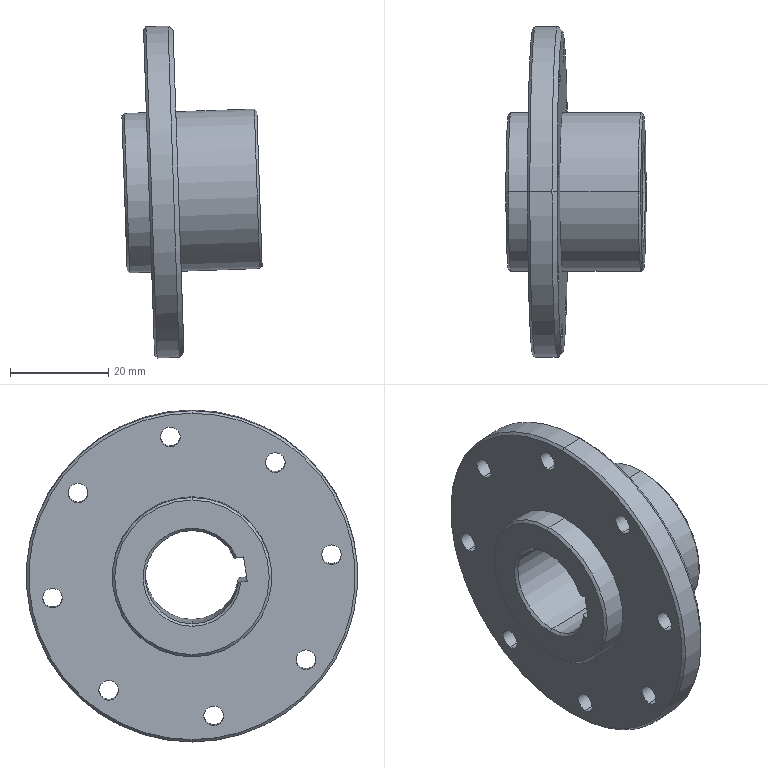Part | STEP file | 2026.6.15-Main Assembly图.sldasm-Part-101 | 1 solid | 46 faces | box 28.549 x 67.5 x 67.614 mm | volume 30514 mm3 | cylinder 25 | cone 14 | plane 7 | commonest cylinder face diameters 4 x16 32.5 x4 19 x3 67.5 x2
STEP:
#1=CARTESIAN_POINT('',(-1623.534,735.086,4084.159));
#2=VERTEX_POINT('',#1);
#3=CARTESIAN_POINT('',(-1625.749,735.086,4149.621));
#4=VERTEX_POINT('',#3);
#5=CARTESIAN_POINT('',(-1624.641,735.086,4116.89));
#6=DIRECTION('',(0.9994,0.,0.03381));
#7=DIRECTION('',(0.03381,0.,-0.9994));
#8=AXIS2_PLACEMENT_3D('',#5,#6,#7);
#9=CIRCLE('',#8,32.75);
#10=EDGE_CURVE('',#2,#4,#9,.T.);
#11=ORIENTED_EDGE('',*,*,#10,.F.);
#12=CARTESIAN_POINT('',(-1624.499,735.086,4083.125));
#13=VERTEX_POINT('',#12);
#14=CARTESIAN_POINT('',(-1623.534,735.086,4084.159));
#15=DIRECTION('',(-0.6828,0.,-0.7306));
#16=VECTOR('',#15,1000.);
#17=LINE('',#14,#16);
#18=EDGE_CURVE('',#2,#13,#17,.T.);
#19=ORIENTED_EDGE('',*,*,#18,.T.);
#20=CARTESIAN_POINT('',(-1626.782,735.086,4150.587));
#21=VERTEX_POINT('',#20);
#22=CARTESIAN_POINT('',(-1625.641,735.086,4116.856));
#23=DIRECTION('',(-0.9994,0.,-0.03381));
#24=DIRECTION('',(0.03381,0.,-0.9994));
#25=AXIS2_PLACEMENT_3D('',#22,#23,#24);
#26=CIRCLE('',#25,33.75);
#27=EDGE_CURVE('',#21,#13,#26,.T.);
#28=ORIENTED_EDGE('',*,*,#27,.F.);
#29=CARTESIAN_POINT('',(-1625.749,735.086,4149.621));
#30=DIRECTION('',(-0.7306,0.,0.6828));
#31=VECTOR('',#30,1000.);
#32=LINE('',#29,#31);
#33=EDGE_CURVE('',#4,#21,#32,.T.);
#34=ORIENTED_EDGE('',*,*,#33,.F.);
#35=EDGE_LOOP('',(#11,#19,#28,#34));
#36=FACE_OUTER_BOUND('',#35,.T.);
#37=CARTESIAN_POINT('',(-1624.641,735.086,4116.89));
#38=DIRECTION('',(-0.9994,0.,-0.03381));
#39=DIRECTION('',(-0.03381,0.,0.9994));
#40=AXIS2_PLACEMENT_3D('',#37,#38,#39);
#41=CONICAL_SURFACE('',#40,32.75,0.7854);
#42=ADVANCED_FACE('',(#36),#41,.T.);
#43=CARTESIAN_POINT('',(-1634.814,735.086,4107.04));
#44=VERTEX_POINT('',#43);
#45=CARTESIAN_POINT('',(-1635.099,725.645,4115.472));
#46=VERTEX_POINT('',#45);
#47=CARTESIAN_POINT('',(-1635.135,735.086,4116.535));
#48=DIRECTION('',(-0.9994,0.,-0.03381));
#49=DIRECTION('',(0.03381,0.,-0.9994));
#50=AXIS2_PLACEMENT_3D('',#47,#48,#49);
#51=CIRCLE('',#50,9.5);
#52=EDGE_CURVE('',#44,#46,#51,.T.);
#53=ORIENTED_EDGE('',*,*,#52,.F.);
#54=CARTESIAN_POINT('',(-1635.297,735.086,4106.524));
#55=VERTEX_POINT('',#54);
#56=CARTESIAN_POINT('',(-1634.814,735.086,4107.04));
#57=DIRECTION('',(-0.6828,0.,-0.7306));
#58=VECTOR('',#57,1000.);
#59=LINE('',#56,#58);
#60=EDGE_CURVE('',#44,#55,#59,.T.);
#61=ORIENTED_EDGE('',*,*,#60,.T.);
#62=CARTESIAN_POINT('',(-1635.602,725.134,4115.534));
#63=VERTEX_POINT('',#62);
#64=CARTESIAN_POINT('',(-1635.635,735.086,4116.518));
#65=DIRECTION('',(0.9994,0.,0.03381));
#66=DIRECTION('',(0.03381,0.,-0.9994));
#67=AXIS2_PLACEMENT_3D('',#64,#65,#66);
#68=CIRCLE('',#67,10.);
#69=EDGE_CURVE('',#63,#55,#68,.T.);
#70=ORIENTED_EDGE('',*,*,#69,.F.);
#71=CARTESIAN_POINT('',(-1635.099,725.645,4115.472));
#72=CARTESIAN_POINT('',(-1635.267,725.475,4115.493));
#73=CARTESIAN_POINT('',(-1635.434,725.305,4115.513));
#74=CARTESIAN_POINT('',(-1635.602,725.134,4115.534));
#75=B_SPLINE_CURVE_WITH_KNOTS('',3,(#71,#72,#73,#74),.UNSPECIFIED.,.F.,.F.,(4,4),(0.,0.0007194),.UNSPECIFIED.);
#76=EDGE_CURVE('',#46,#63,#75,.T.);
#77=ORIENTED_EDGE('',*,*,#76,.F.);
#78=EDGE_LOOP('',(#53,#61,#70,#77));
#79=FACE_OUTER_BOUND('',#78,.T.);
#80=CARTESIAN_POINT('',(-1635.135,735.086,4116.535));
#81=DIRECTION('',(-0.9994,0.,-0.03381));
#82=DIRECTION('',(-0.03381,0.,0.9994));
#83=AXIS2_PLACEMENT_3D('',#80,#81,#82);
#84=CONICAL_SURFACE('',#83,9.5,0.7854);
#85=ADVANCED_FACE('',(#79),#84,.F.);
#86=ORIENTED_EDGE('',*,*,#60,.F.);
#87=CARTESIAN_POINT('',(-1635.457,735.086,4126.03));
#88=VERTEX_POINT('',#87);
#89=CARTESIAN_POINT('',(-1635.135,735.086,4116.535));
#90=DIRECTION('',(-0.9994,0.,-0.03381));
#91=DIRECTION('',(0.03381,0.,-0.9994));
#92=AXIS2_PLACEMENT_3D('',#89,#90,#91);
#93=CIRCLE('',#92,9.5);
#94=EDGE_CURVE('',#88,#44,#93,.T.);
#95=ORIENTED_EDGE('',*,*,#94,.F.);
#96=CARTESIAN_POINT('',(-1635.973,735.086,4126.512));
#97=VERTEX_POINT('',#96);
#98=CARTESIAN_POINT('',(-1635.457,735.086,4126.03));
#99=DIRECTION('',(-0.7306,0.,0.6828));
#100=VECTOR('',#99,1000.);
#101=LINE('',#98,#100);
#102=EDGE_CURVE('',#88,#97,#101,.T.);
#103=ORIENTED_EDGE('',*,*,#102,.T.);
#104=CARTESIAN_POINT('',(-1635.635,735.086,4116.518));
#105=DIRECTION('',(0.9994,0.,0.03381));
#106=DIRECTION('',(0.03381,0.,-0.9994));
#107=AXIS2_PLACEMENT_3D('',#104,#105,#106);
#108=CIRCLE('',#107,10.);
#109=EDGE_CURVE('',#55,#97,#108,.T.);
#110=ORIENTED_EDGE('',*,*,#109,.F.);
#111=EDGE_LOOP('',(#86,#95,#103,#110));
#112=FACE_OUTER_BOUND('',#111,.T.);
#113=CARTESIAN_POINT('',(-1635.135,735.086,4116.535));
#114=DIRECTION('',(-0.9994,0.,-0.03381));
#115=DIRECTION('',(-0.03381,0.,0.9994));
#116=AXIS2_PLACEMENT_3D('',#113,#114,#115);
#117=CONICAL_SURFACE('',#116,9.5,0.7854);
#118=ADVANCED_FACE('',(#112),#117,.F.);
#119=CARTESIAN_POINT('',(-1636.168,735.086,4132.259));
#120=VERTEX_POINT('',#119);
#121=CARTESIAN_POINT('',(-1635.102,735.086,4100.777));
#122=VERTEX_POINT('',#121);
#123=CARTESIAN_POINT('',(-1635.635,735.086,4116.518));
#124=DIRECTION('',(-0.9994,0.,-0.03381));
#125=DIRECTION('',(0.03381,0.,-0.9994));
#126=AXIS2_PLACEMENT_3D('',#123,#124,#125);
#127=CIRCLE('',#126,15.75);
#128=EDGE_CURVE('',#120,#122,#127,.T.);
#129=ORIENTED_EDGE('',*,*,#128,.F.);
#130=CARTESIAN_POINT('',(-1635.685,735.086,4132.776));
#131=VERTEX_POINT('',#130);
#132=CARTESIAN_POINT('',(-1635.685,735.086,4132.776));
#133=DIRECTION('',(0.6828,0.,0.7306));
#134=VECTOR('',#133,1000.);
#135=LINE('',#132,#134);
#136=EDGE_CURVE('',#120,#131,#135,.T.);
#137=ORIENTED_EDGE('',*,*,#136,.T.);
#138=CARTESIAN_POINT('',(-1634.586,735.086,4100.294));
#139=VERTEX_POINT('',#138);
#140=CARTESIAN_POINT('',(-1635.135,735.086,4116.535));
#141=DIRECTION('',(0.9994,0.,0.03381));
#142=DIRECTION('',(0.03381,0.,-0.9994));
#143=AXIS2_PLACEMENT_3D('',#140,#141,#142);
#144=CIRCLE('',#143,16.25);
#145=EDGE_CURVE('',#139,#131,#144,.T.);
#146=ORIENTED_EDGE('',*,*,#145,.F.);
#147=CARTESIAN_POINT('',(-1634.586,735.086,4100.294));
#148=DIRECTION('',(0.7306,0.,-0.6828));
#149=VECTOR('',#148,1000.);
#150=LINE('',#147,#149);
#151=EDGE_CURVE('',#122,#139,#150,.T.);
#152=ORIENTED_EDGE('',*,*,#151,.F.);
#153=EDGE_LOOP('',(#129,#137,#146,#152));
#154=FACE_OUTER_BOUND('',#153,.T.);
#155=CARTESIAN_POINT('',(-1635.135,735.086,4116.535));
#156=DIRECTION('',(0.9994,0.,0.03381));
#157=DIRECTION('',(0.03381,0.,-0.9994));
#158=AXIS2_PLACEMENT_3D('',#155,#156,#157);
#159=CONICAL_SURFACE('',#158,16.25,0.7854);
#160=ADVANCED_FACE('',(#154),#159,.T.);
#161=CARTESIAN_POINT('',(-1631.762,735.086,4149.918));
#162=VERTEX_POINT('',#161);
#163=CARTESIAN_POINT('',(-1629.514,735.086,4083.456));
#164=VERTEX_POINT('',#163);
#165=CARTESIAN_POINT('',(-1630.638,735.086,4116.687));
#166=DIRECTION('',(-0.9994,0.,-0.03381));
#167=DIRECTION('',(0.03381,0.,-0.9994));
#168=AXIS2_PLACEMENT_3D('',#165,#166,#167);
#169=CIRCLE('',#168,33.25);
#170=EDGE_CURVE('',#162,#164,#169,.T.);
#171=ORIENTED_EDGE('',*,*,#170,.F.);
#172=CARTESIAN_POINT('',(-1631.279,735.086,4150.435));
#173=VERTEX_POINT('',#172);
#174=CARTESIAN_POINT('',(-1631.279,735.086,4150.435));
#175=DIRECTION('',(0.6828,0.,0.7306));
#176=VECTOR('',#175,1000.);
#177=LINE('',#174,#176);
#178=EDGE_CURVE('',#162,#173,#177,.T.);
#179=ORIENTED_EDGE('',*,*,#178,.T.);
#180=CARTESIAN_POINT('',(-1628.997,735.086,4082.973));
#181=VERTEX_POINT('',#180);
#182=CARTESIAN_POINT('',(-1630.138,735.086,4116.704));
#183=DIRECTION('',(0.9994,0.,0.03381));
#184=DIRECTION('',(0.03381,0.,-0.9994));
#185=AXIS2_PLACEMENT_3D('',#182,#183,#184);
#186=CIRCLE('',#185,33.75);
#187=EDGE_CURVE('',#181,#173,#186,.T.);
#188=ORIENTED_EDGE('',*,*,#187,.F.);
#189=CARTESIAN_POINT('',(-1628.997,735.086,4082.973));
#190=DIRECTION('',(0.7306,0.,-0.6828));
#191=VECTOR('',#190,1000.);
#192=LINE('',#189,#191);
#193=EDGE_CURVE('',#164,#181,#192,.T.);
#194=ORIENTED_EDGE('',*,*,#193,.F.);
#195=EDGE_LOOP('',(#171,#179,#188,#194));
#196=FACE_OUTER_BOUND('',#195,.T.);
#197=CARTESIAN_POINT('',(-1630.138,735.086,4116.704));
#198=DIRECTION('',(0.9994,0.,0.03381));
#199=DIRECTION('',(0.03381,0.,-0.9994));
#200=AXIS2_PLACEMENT_3D('',#197,#198,#199);
#201=CONICAL_SURFACE('',#200,33.75,0.7854);
#202=ADVANCED_FACE('',(#196),#201,.T.);
#203=CARTESIAN_POINT('',(-1607.618,735.086,4101.707));
#204=VERTEX_POINT('',#203);
#205=CARTESIAN_POINT('',(-1608.683,735.086,4133.189));
#206=VERTEX_POINT('',#205);
#207=CARTESIAN_POINT('',(-1608.151,735.086,4117.448));
#208=DIRECTION('',(0.9994,0.,0.03381));
#209=DIRECTION('',(0.03381,0.,-0.9994));
#210=AXIS2_PLACEMENT_3D('',#207,#208,#209);
#211=CIRCLE('',#210,15.75);
#212=EDGE_CURVE('',#204,#206,#211,.T.);
#213=ORIENTED_EDGE('',*,*,#212,.F.);
#214=CARTESIAN_POINT('',(-1608.101,735.086,4101.19));
#215=VERTEX_POINT('',#214);
#216=CARTESIAN_POINT('',(-1607.618,735.086,4101.707));
#217=DIRECTION('',(-0.6828,0.,-0.7306));
#218=VECTOR('',#217,1000.);
#219=LINE('',#216,#218);
#220=EDGE_CURVE('',#204,#215,#219,.T.);
#221=ORIENTED_EDGE('',*,*,#220,.T.);
#222=CARTESIAN_POINT('',(-1609.2,735.086,4133.672));
#223=VERTEX_POINT('',#222);
#224=CARTESIAN_POINT('',(-1608.65,735.086,4117.431));
#225=DIRECTION('',(-0.9994,0.,-0.03381));
#226=DIRECTION('',(0.03381,0.,-0.9994));
#227=AXIS2_PLACEMENT_3D('',#224,#225,#226);
#228=CIRCLE('',#227,16.25);
#229=EDGE_CURVE('',#223,#215,#228,.T.);
#230=ORIENTED_EDGE('',*,*,#229,.F.);
#231=CARTESIAN_POINT('',(-1608.683,735.086,4133.189));
#232=DIRECTION('',(-0.7306,0.,0.6828));
#233=VECTOR('',#232,1000.);
#234=LINE('',#231,#233);
#235=EDGE_CURVE('',#206,#223,#234,.T.);
#236=ORIENTED_EDGE('',*,*,#235,.F.);
#237=EDGE_LOOP('',(#213,#221,#230,#236));
#238=FACE_OUTER_BOUND('',#237,.T.);
#239=CARTESIAN_POINT('',(-1608.151,735.086,4117.448));
#240=DIRECTION('',(-0.9994,0.,-0.03381));
#241=DIRECTION('',(-0.03381,0.,0.9994));
#242=AXIS2_PLACEMENT_3D('',#239,#240,#241);
#243=CONICAL_SURFACE('',#242,15.75,0.7854);
#244=ADVANCED_FACE('',(#238),#243,.T.);
#245=CARTESIAN_POINT('',(-1608.972,735.086,4126.926));
#246=VERTEX_POINT('',#245);
#247=CARTESIAN_POINT('',(-1608.782,726.413,4121.306));
#248=VERTEX_POINT('',#247);
#249=CARTESIAN_POINT('',(-1608.65,735.086,4117.431));
#250=DIRECTION('',(0.9994,0.,0.03381));
#251=DIRECTION('',(0.03381,0.,-0.9994));
#252=AXIS2_PLACEMENT_3D('',#249,#250,#251);
#253=CIRCLE('',#252,9.5);
#254=EDGE_CURVE('',#246,#248,#253,.T.);
#255=ORIENTED_EDGE('',*,*,#254,.F.);
#256=CARTESIAN_POINT('',(-1608.489,735.086,4127.442));
#257=VERTEX_POINT('',#256);
#258=CARTESIAN_POINT('',(-1608.489,735.086,4127.442));
#259=DIRECTION('',(0.6828,0.,0.7306));
#260=VECTOR('',#259,1000.);
#261=LINE('',#258,#260);
#262=EDGE_CURVE('',#246,#257,#261,.T.);
#263=ORIENTED_EDGE('',*,*,#262,.T.);
#264=CARTESIAN_POINT('',(-1608.285,725.902,4121.402));
#265=VERTEX_POINT('',#264);
#266=CARTESIAN_POINT('',(-1608.151,735.086,4117.448));
#267=DIRECTION('',(-0.9994,0.,-0.03381));
#268=DIRECTION('',(0.03381,0.,-0.9994));
#269=AXIS2_PLACEMENT_3D('',#266,#267,#268);
#270=CIRCLE('',#269,10.);
#271=EDGE_CURVE('',#265,#257,#270,.T.);
#272=ORIENTED_EDGE('',*,*,#271,.F.);
#273=CARTESIAN_POINT('',(-1608.782,726.413,4121.306));
#274=CARTESIAN_POINT('',(-1608.616,726.242,4121.338));
#275=CARTESIAN_POINT('',(-1608.45,726.072,4121.37));
#276=CARTESIAN_POINT('',(-1608.285,725.902,4121.402));
#277=B_SPLINE_CURVE_WITH_KNOTS('',3,(#273,#274,#275,#276),.UNSPECIFIED.,.F.,.F.,(4,4),(0.,0.0007194),.UNSPECIFIED.);
#278=EDGE_CURVE('',#248,#265,#277,.T.);
#279=ORIENTED_EDGE('',*,*,#278,.F.);
#280=EDGE_LOOP('',(#255,#263,#272,#279));
#281=FACE_OUTER_BOUND('',#280,.T.);
#282=CARTESIAN_POINT('',(-1608.151,735.086,4117.448));
#283=DIRECTION('',(0.9994,0.,0.03381));
#284=DIRECTION('',(0.03381,0.,-0.9994));
#285=AXIS2_PLACEMENT_3D('',#282,#283,#284);
#286=CONICAL_SURFACE('',#285,10.,0.7854);
#287=ADVANCED_FACE('',(#281),#286,.F.);
#288=ORIENTED_EDGE('',*,*,#262,.F.);
#289=CARTESIAN_POINT('',(-1608.329,735.086,4107.936));
#290=VERTEX_POINT('',#289);
#291=CARTESIAN_POINT('',(-1608.65,735.086,4117.431));
#292=DIRECTION('',(0.9994,0.,0.03381));
#293=DIRECTION('',(0.03381,0.,-0.9994));
#294=AXIS2_PLACEMENT_3D('',#291,#292,#293);
#295=CIRCLE('',#294,9.5);
#296=EDGE_CURVE('',#290,#246,#295,.T.);
#297=ORIENTED_EDGE('',*,*,#296,.F.);
#298=CARTESIAN_POINT('',(-1607.813,735.086,4107.454));
#299=VERTEX_POINT('',#298);
#300=CARTESIAN_POINT('',(-1607.813,735.086,4107.454));
#301=DIRECTION('',(0.7306,0.,-0.6828));
#302=VECTOR('',#301,1000.);
#303=LINE('',#300,#302);
#304=EDGE_CURVE('',#290,#299,#303,.T.);
#305=ORIENTED_EDGE('',*,*,#304,.T.);
#306=CARTESIAN_POINT('',(-1608.151,735.086,4117.448));
#307=DIRECTION('',(-0.9994,0.,-0.03381));
#308=DIRECTION('',(0.03381,0.,-0.9994));
#309=AXIS2_PLACEMENT_3D('',#306,#307,#308);
#310=CIRCLE('',#309,10.);
#311=EDGE_CURVE('',#257,#299,#310,.T.);
#312=ORIENTED_EDGE('',*,*,#311,.F.);
#313=EDGE_LOOP('',(#288,#297,#305,#312));
#314=FACE_OUTER_BOUND('',#313,.T.);
#315=CARTESIAN_POINT('',(-1608.151,735.086,4117.448));
#316=DIRECTION('',(0.9994,0.,0.03381));
#317=DIRECTION('',(0.03381,0.,-0.9994));
#318=AXIS2_PLACEMENT_3D('',#315,#316,#317);
#319=CONICAL_SURFACE('',#318,10.,0.7854);
#320=ADVANCED_FACE('',(#314),#319,.F.);
#321=ORIENTED_EDGE('',*,*,#27,.T.);
#322=CARTESIAN_POINT('',(-1623.5,735.086,4083.159));
#323=DIRECTION('',(-0.9994,0.,-0.03381));
#324=VECTOR('',#323,1000.);
#325=LINE('',#322,#324);
#326=EDGE_CURVE('',#13,#181,#325,.T.);
#327=ORIENTED_EDGE('',*,*,#326,.T.);
#328=ORIENTED_EDGE('',*,*,#187,.T.);
#329=CARTESIAN_POINT('',(-1625.783,735.086,4150.621));
#330=DIRECTION('',(-0.9994,0.,-0.03381));
#331=VECTOR('',#330,1000.);
#332=LINE('',#329,#331);
#333=EDGE_CURVE('',#21,#173,#332,.T.);
#334=ORIENTED_EDGE('',*,*,#333,.F.);
#335=EDGE_LOOP('',(#321,#327,#328,#334));
#336=FACE_OUTER_BOUND('',#335,.T.);
#337=CARTESIAN_POINT('',(-1624.641,735.086,4116.89));
#338=DIRECTION('',(-0.9994,0.,-0.03381));
#339=DIRECTION('',(-0.03381,0.,0.9994));
#340=AXIS2_PLACEMENT_3D('',#337,#338,#339);
#341=CYLINDRICAL_SURFACE('',#340,33.75);
#342=ADVANCED_FACE('',(#336),#341,.T.);
#343=CARTESIAN_POINT('',(-1625.358,718.117,4138.086));
#344=VERTEX_POINT('',#343);
#345=CARTESIAN_POINT('',(-1625.494,718.117,4142.084));
#346=VERTEX_POINT('',#345);
#347=CARTESIAN_POINT('',(-1625.426,718.117,4140.085));
#348=DIRECTION('',(-0.9994,0.,-0.03381));
#349=DIRECTION('',(-0.03341,0.1535,0.9876));
#350=AXIS2_PLACEMENT_3D('',#347,#348,#349);
#351=CIRCLE('',#350,2.);
#352=EDGE_CURVE('',#344,#346,#351,.T.);
#353=ORIENTED_EDGE('',*,*,#352,.F.);
#354=CARTESIAN_POINT('',(-1631.355,718.117,4137.883));
#355=VERTEX_POINT('',#354);
#356=CARTESIAN_POINT('',(-1625.358,718.117,4138.086));
#357=DIRECTION('',(-0.9994,0.,-0.03381));
#358=VECTOR('',#357,1000.);
#359=LINE('',#356,#358);
#360=EDGE_CURVE('',#344,#355,#359,.T.);
#361=ORIENTED_EDGE('',*,*,#360,.T.);
#362=CARTESIAN_POINT('',(-1631.49,718.117,4141.881));
#363=VERTEX_POINT('',#362);
#364=CARTESIAN_POINT('',(-1631.423,718.117,4139.882));
#365=DIRECTION('',(-0.9994,0.,-0.03381));
#366=DIRECTION('',(-0.03341,0.1535,0.9876));
#367=AXIS2_PLACEMENT_3D('',#364,#365,#366);
#368=CIRCLE('',#367,2.);
#369=EDGE_CURVE('',#355,#363,#368,.T.);
#370=ORIENTED_EDGE('',*,*,#369,.T.);
#371=CARTESIAN_POINT('',(-1625.494,718.117,4142.084));
#372=DIRECTION('',(-0.9994,0.,-0.03381));
#373=VECTOR('',#372,1000.);
#374=LINE('',#371,#373);
#375=EDGE_CURVE('',#346,#363,#374,.T.);
#376=ORIENTED_EDGE('',*,*,#375,.F.);
#377=EDGE_LOOP('',(#353,#361,#370,#376));
#378=FACE_OUTER_BOUND('',#377,.T.);
#379=CARTESIAN_POINT('',(-1625.426,718.117,4140.085));
#380=DIRECTION('',(-0.9994,0.,-0.03381));
#381=DIRECTION('',(-0.03381,0.,0.9994));
#382=AXIS2_PLACEMENT_3D('',#379,#380,#381);
#383=CYLINDRICAL_SURFACE('',#382,2.);
#384=ADVANCED_FACE('',(#378),#383,.F.);
#385=CARTESIAN_POINT('',(-1625.283,758.294,4135.848));
#386=VERTEX_POINT('',#385);
#387=CARTESIAN_POINT('',(-1625.147,758.294,4131.85));
#388=VERTEX_POINT('',#387);
#389=CARTESIAN_POINT('',(-1625.215,758.294,4133.849));
#390=DIRECTION('',(0.9994,0.,0.03381));
#391=DIRECTION('',(-0.03341,0.1535,0.9876));
#392=AXIS2_PLACEMENT_3D('',#389,#390,#391);
#393=CIRCLE('',#392,2.);
#394=EDGE_CURVE('',#386,#388,#393,.T.);
#395=ORIENTED_EDGE('',*,*,#394,.T.);
#396=CARTESIAN_POINT('',(-1631.144,758.294,4131.647));
#397=VERTEX_POINT('',#396);
#398=CARTESIAN_POINT('',(-1625.147,758.294,4131.85));
#399=DIRECTION('',(-0.9994,0.,-0.03381));
#400=VECTOR('',#399,1000.);
#401=LINE('',#398,#400);
#402=EDGE_CURVE('',#388,#397,#401,.T.);
#403=ORIENTED_EDGE('',*,*,#402,.T.);
#404=CARTESIAN_POINT('',(-1631.279,758.294,4135.645));
#405=VERTEX_POINT('',#404);
#406=CARTESIAN_POINT('',(-1631.212,758.294,4133.646));
#407=DIRECTION('',(0.9994,0.,0.03381));
#408=DIRECTION('',(-0.03341,0.1535,0.9876));
#409=AXIS2_PLACEMENT_3D('',#406,#407,#408);
#410=CIRCLE('',#409,2.);
#411=EDGE_CURVE('',#405,#397,#410,.T.);
#412=ORIENTED_EDGE('',*,*,#411,.F.);
#413=CARTESIAN_POINT('',(-1625.283,758.294,4135.848));
#414=DIRECTION('',(-0.9994,0.,-0.03381));
#415=VECTOR('',#414,1000.);
#416=LINE('',#413,#415);
#417=EDGE_CURVE('',#386,#405,#416,.T.);
#418=ORIENTED_EDGE('',*,*,#417,.F.);
#419=EDGE_LOOP('',(#395,#403,#412,#418));
#420=FACE_OUTER_BOUND('',#419,.T.);
#421=CARTESIAN_POINT('',(-1625.215,758.294,4133.849));
#422=DIRECTION('',(-0.9994,0.,-0.03381));
#423=DIRECTION('',(-0.03381,0.,0.9994));
#424=AXIS2_PLACEMENT_3D('',#421,#422,#423);
#425=CYLINDRICAL_SURFACE('',#424,2.);
#426=ADVANCED_FACE('',(#420),#425,.F.);
#427=CARTESIAN_POINT('',(-1624.424,763.495,4110.481));
#428=VERTEX_POINT('',#427);
#429=CARTESIAN_POINT('',(-1624.56,763.495,4114.479));
#430=VERTEX_POINT('',#429);
#431=CARTESIAN_POINT('',(-1624.492,763.495,4112.48));
#432=DIRECTION('',(-0.9994,0.,-0.03381));
#433=DIRECTION('',(-0.03341,0.1535,0.9876));
#434=AXIS2_PLACEMENT_3D('',#431,#432,#433);
#435=CIRCLE('',#434,2.);
#436=EDGE_CURVE('',#428,#430,#435,.T.);
#437=ORIENTED_EDGE('',*,*,#436,.F.);
#438=CARTESIAN_POINT('',(-1630.421,763.495,4110.278));
#439=VERTEX_POINT('',#438);
#440=CARTESIAN_POINT('',(-1624.424,763.495,4110.481));
#441=DIRECTION('',(-0.9994,0.,-0.03381));
#442=VECTOR('',#441,1000.);
#443=LINE('',#440,#442);
#444=EDGE_CURVE('',#428,#439,#443,.T.);
#445=ORIENTED_EDGE('',*,*,#444,.T.);
#446=CARTESIAN_POINT('',(-1630.556,763.495,4114.276));
#447=VERTEX_POINT('',#446);
#448=CARTESIAN_POINT('',(-1630.489,763.495,4112.277));
#449=DIRECTION('',(-0.9994,0.,-0.03381));
#450=DIRECTION('',(-0.03341,0.1535,0.9876));
#451=AXIS2_PLACEMENT_3D('',#448,#449,#450);
#452=CIRCLE('',#451,2.);
#453=EDGE_CURVE('',#439,#447,#452,.T.);
#454=ORIENTED_EDGE('',*,*,#453,.T.);
#455=CARTESIAN_POINT('',(-1624.56,763.495,4114.479));
#456=DIRECTION('',(-0.9994,0.,-0.03381));
#457=VECTOR('',#456,1000.);
#458=LINE('',#455,#457);
#459=EDGE_CURVE('',#430,#447,#458,.T.);
#460=ORIENTED_EDGE('',*,*,#459,.F.);
#461=EDGE_LOOP('',(#437,#445,#454,#460));
#462=FACE_OUTER_BOUND('',#461,.T.);
#463=CARTESIAN_POINT('',(-1624.492,763.495,4112.48));
#464=DIRECTION('',(-0.9994,0.,-0.03381));
#465=DIRECTION('',(-0.03381,0.,0.9994));
#466=AXIS2_PLACEMENT_3D('',#463,#464,#465);
#467=CYLINDRICAL_SURFACE('',#466,2.);
#468=ADVANCED_FACE('',(#462),#467,.F.);
#469=CARTESIAN_POINT('',(-1623.789,752.054,4091.696));
#470=VERTEX_POINT('',#469);
#471=CARTESIAN_POINT('',(-1623.924,752.054,4095.694));
#472=VERTEX_POINT('',#471);
#473=CARTESIAN_POINT('',(-1623.857,752.054,4093.695));
#474=DIRECTION('',(-0.9994,0.,-0.03381));
#475=DIRECTION('',(-0.03341,0.1535,0.9876));
#476=AXIS2_PLACEMENT_3D('',#473,#474,#475);
#477=CIRCLE('',#476,2.);
#478=EDGE_CURVE('',#470,#472,#477,.T.);
#479=ORIENTED_EDGE('',*,*,#478,.F.);
#480=CARTESIAN_POINT('',(-1629.785,752.054,4091.493));
#481=VERTEX_POINT('',#480);
#482=CARTESIAN_POINT('',(-1623.789,752.054,4091.696));
#483=DIRECTION('',(-0.9994,0.,-0.03381));
#484=VECTOR('',#483,1000.);
#485=LINE('',#482,#484);
#486=EDGE_CURVE('',#470,#481,#485,.T.);
#487=ORIENTED_EDGE('',*,*,#486,.T.);
#488=CARTESIAN_POINT('',(-1629.921,752.054,4095.491));
#489=VERTEX_POINT('',#488);
#490=CARTESIAN_POINT('',(-1629.853,752.054,4093.492));
#491=DIRECTION('',(-0.9994,0.,-0.03381));
#492=DIRECTION('',(-0.03341,0.1535,0.9876));
#493=AXIS2_PLACEMENT_3D('',#490,#491,#492);
#494=CIRCLE('',#493,2.);
#495=EDGE_CURVE('',#481,#489,#494,.T.);
#496=ORIENTED_EDGE('',*,*,#495,.T.);
#497=CARTESIAN_POINT('',(-1623.924,752.054,4095.694));
#498=DIRECTION('',(-0.9994,0.,-0.03381));
#499=VECTOR('',#498,1000.);
#500=LINE('',#497,#499);
#501=EDGE_CURVE('',#472,#489,#500,.T.);
#502=ORIENTED_EDGE('',*,*,#501,.F.);
#503=EDGE_LOOP('',(#479,#487,#496,#502));
#504=FACE_OUTER_BOUND('',#503,.T.);
#505=CARTESIAN_POINT('',(-1623.857,752.054,4093.695));
#506=DIRECTION('',(-0.9994,0.,-0.03381));
#507=DIRECTION('',(-0.03381,0.,0.9994));
#508=AXIS2_PLACEMENT_3D('',#505,#506,#507);
#509=CYLINDRICAL_SURFACE('',#508,2.);
#510=ADVANCED_FACE('',(#504),#509,.F.);
#511=CARTESIAN_POINT('',(-1623.613,730.673,4086.498));
#512=VERTEX_POINT('',#511);
#513=CARTESIAN_POINT('',(-1623.748,730.673,4090.496));
#514=VERTEX_POINT('',#513);
#515=CARTESIAN_POINT('',(-1623.681,730.673,4088.497));
#516=DIRECTION('',(-0.9994,0.,-0.03381));
#517=DIRECTION('',(-0.03341,0.1535,0.9876));
#518=AXIS2_PLACEMENT_3D('',#515,#516,#517);
#519=CIRCLE('',#518,2.);
#520=EDGE_CURVE('',#512,#514,#519,.T.);
#521=ORIENTED_EDGE('',*,*,#520,.F.);
#522=CARTESIAN_POINT('',(-1629.61,730.673,4086.295));
#523=VERTEX_POINT('',#522);
#524=CARTESIAN_POINT('',(-1623.613,730.673,4086.498));
#525=DIRECTION('',(-0.9994,0.,-0.03381));
#526=VECTOR('',#525,1000.);
#527=LINE('',#524,#526);
#528=EDGE_CURVE('',#512,#523,#527,.T.);
#529=ORIENTED_EDGE('',*,*,#528,.T.);
#530=CARTESIAN_POINT('',(-1629.745,730.673,4090.293));
#531=VERTEX_POINT('',#530);
#532=CARTESIAN_POINT('',(-1629.677,730.673,4088.294));
#533=DIRECTION('',(-0.9994,0.,-0.03381));
#534=DIRECTION('',(-0.03341,0.1535,0.9876));
#535=AXIS2_PLACEMENT_3D('',#532,#533,#534);
#536=CIRCLE('',#535,2.);
#537=EDGE_CURVE('',#523,#531,#536,.T.);
#538=ORIENTED_EDGE('',*,*,#537,.T.);
#539=CARTESIAN_POINT('',(-1623.748,730.673,4090.496));
#540=DIRECTION('',(-0.9994,0.,-0.03381));
#541=VECTOR('',#540,1000.);
#542=LINE('',#539,#541);
#543=EDGE_CURVE('',#514,#531,#542,.T.);
#544=ORIENTED_EDGE('',*,*,#543,.F.);
#545=EDGE_LOOP('',(#521,#529,#538,#544));
#546=FACE_OUTER_BOUND('',#545,.T.);
#547=CARTESIAN_POINT('',(-1623.681,730.673,4088.497));
#548=DIRECTION('',(-0.9994,0.,-0.03381));
#549=DIRECTION('',(-0.03381,0.,0.9994));
#550=AXIS2_PLACEMENT_3D('',#547,#548,#549);
#551=CYLINDRICAL_SURFACE('',#550,2.);
#552=ADVANCED_FACE('',(#546),#551,.F.);
#553=CARTESIAN_POINT('',(-1624.,711.877,4097.932));
#554=VERTEX_POINT('',#553);
#555=CARTESIAN_POINT('',(-1624.135,711.877,4101.93));
#556=VERTEX_POINT('',#555);
#557=CARTESIAN_POINT('',(-1624.068,711.877,4099.931));
#558=DIRECTION('',(-0.9994,0.,-0.03381));
#559=DIRECTION('',(-0.03341,0.1535,0.9876));
#560=AXIS2_PLACEMENT_3D('',#557,#558,#559);
#561=CIRCLE('',#560,2.);
#562=EDGE_CURVE('',#554,#556,#561,.T.);
#563=ORIENTED_EDGE('',*,*,#562,.F.);
#564=CARTESIAN_POINT('',(-1629.996,711.877,4097.73));
#565=VERTEX_POINT('',#564);
#566=CARTESIAN_POINT('',(-1624.,711.877,4097.932));
#567=DIRECTION('',(-0.9994,0.,-0.03381));
#568=VECTOR('',#567,1000.);
#569=LINE('',#566,#568);
#570=EDGE_CURVE('',#554,#565,#569,.T.);
#571=ORIENTED_EDGE('',*,*,#570,.T.);
#572=CARTESIAN_POINT('',(-1630.132,711.877,4101.727));
#573=VERTEX_POINT('',#572);
#574=CARTESIAN_POINT('',(-1630.064,711.877,4099.728));
#575=DIRECTION('',(-0.9994,0.,-0.03381));
#576=DIRECTION('',(-0.03341,0.1535,0.9876));
#577=AXIS2_PLACEMENT_3D('',#574,#575,#576);
#578=CIRCLE('',#577,2.);
#579=EDGE_CURVE('',#565,#573,#578,.T.);
#580=ORIENTED_EDGE('',*,*,#579,.T.);
#581=CARTESIAN_POINT('',(-1624.135,711.877,4101.93));
#582=DIRECTION('',(-0.9994,0.,-0.03381));
#583=VECTOR('',#582,1000.);
#584=LINE('',#581,#583);
#585=EDGE_CURVE('',#556,#573,#584,.T.);
#586=ORIENTED_EDGE('',*,*,#585,.F.);
#587=EDGE_LOOP('',(#563,#571,#580,#586));
#588=FACE_OUTER_BOUND('',#587,.T.);
#589=CARTESIAN_POINT('',(-1624.068,711.877,4099.931));
#590=DIRECTION('',(-0.9994,0.,-0.03381));
#591=DIRECTION('',(-0.03381,0.,0.9994));
#592=AXIS2_PLACEMENT_3D('',#589,#590,#591);
#593=CYLINDRICAL_SURFACE('',#592,2.);
#594=ADVANCED_FACE('',(#588),#593,.F.);
#595=CARTESIAN_POINT('',(-1624.723,706.676,4119.301));
#596=VERTEX_POINT('',#595);
#597=CARTESIAN_POINT('',(-1624.858,706.676,4123.299));
#598=VERTEX_POINT('',#597);
#599=CARTESIAN_POINT('',(-1624.79,706.676,4121.3));
#600=DIRECTION('',(-0.9994,0.,-0.03381));
#601=DIRECTION('',(-0.03341,0.1535,0.9876));
#602=AXIS2_PLACEMENT_3D('',#599,#600,#601);
#603=CIRCLE('',#602,2.);
#604=EDGE_CURVE('',#596,#598,#603,.T.);
#605=ORIENTED_EDGE('',*,*,#604,.F.);
#606=CARTESIAN_POINT('',(-1630.719,706.676,4119.098));
#607=VERTEX_POINT('',#606);
#608=CARTESIAN_POINT('',(-1624.723,706.676,4119.301));
#609=DIRECTION('',(-0.9994,0.,-0.03381));
#610=VECTOR('',#609,1000.);
#611=LINE('',#608,#610);
#612=EDGE_CURVE('',#596,#607,#611,.T.);
#613=ORIENTED_EDGE('',*,*,#612,.T.);
#614=CARTESIAN_POINT('',(-1630.855,706.676,4123.096));
#615=VERTEX_POINT('',#614);
#616=CARTESIAN_POINT('',(-1630.787,706.676,4121.097));
#617=DIRECTION('',(-0.9994,0.,-0.03381));
#618=DIRECTION('',(-0.03341,0.1535,0.9876));
#619=AXIS2_PLACEMENT_3D('',#616,#617,#618);
#620=CIRCLE('',#619,2.);
#621=EDGE_CURVE('',#607,#615,#620,.T.);
#622=ORIENTED_EDGE('',*,*,#621,.T.);
#623=CARTESIAN_POINT('',(-1624.858,706.676,4123.299));
#624=DIRECTION('',(-0.9994,0.,-0.03381));
#625=VECTOR('',#624,1000.);
#626=LINE('',#623,#625);
#627=EDGE_CURVE('',#598,#615,#626,.T.);
#628=ORIENTED_EDGE('',*,*,#627,.F.);
#629=EDGE_LOOP('',(#605,#613,#622,#628));
#630=FACE_OUTER_BOUND('',#629,.T.);
#631=CARTESIAN_POINT('',(-1624.79,706.676,4121.3));
#632=DIRECTION('',(-0.9994,0.,-0.03381));
#633=DIRECTION('',(-0.03381,0.,0.9994));
#634=AXIS2_PLACEMENT_3D('',#631,#632,#633);
#635=CYLINDRICAL_SURFACE('',#634,2.);
#636=ADVANCED_FACE('',(#630),#635,.F.);
#637=CARTESIAN_POINT('',(-1625.534,739.498,4143.284));
#638=VERTEX_POINT('',#637);
#639=CARTESIAN_POINT('',(-1625.67,739.498,4147.282));
#640=VERTEX_POINT('',#639);
#641=CARTESIAN_POINT('',(-1625.602,739.498,4145.283));
#642=DIRECTION('',(-0.9994,0.,-0.03381));
#643=DIRECTION('',(-0.03341,0.1535,0.9876));
#644=AXIS2_PLACEMENT_3D('',#641,#642,#643);
#645=CIRCLE('',#644,2.);
#646=EDGE_CURVE('',#638,#640,#645,.T.);
#647=ORIENTED_EDGE('',*,*,#646,.F.);
#648=CARTESIAN_POINT('',(-1631.531,739.498,4143.081));
#649=VERTEX_POINT('',#648);
#650=CARTESIAN_POINT('',(-1625.534,739.498,4143.284));
#651=DIRECTION('',(-0.9994,0.,-0.03381));
#652=VECTOR('',#651,1000.);
#653=LINE('',#650,#652);
#654=EDGE_CURVE('',#638,#649,#653,.T.);
#655=ORIENTED_EDGE('',*,*,#654,.T.);
#656=CARTESIAN_POINT('',(-1631.666,739.498,4147.079));
#657=VERTEX_POINT('',#656);
#658=CARTESIAN_POINT('',(-1631.598,739.498,4145.08));
#659=DIRECTION('',(-0.9994,0.,-0.03381));
#660=DIRECTION('',(-0.03341,0.1535,0.9876));
#661=AXIS2_PLACEMENT_3D('',#658,#659,#660);
#662=CIRCLE('',#661,2.);
#663=EDGE_CURVE('',#649,#657,#662,.T.);
#664=ORIENTED_EDGE('',*,*,#663,.T.);
#665=CARTESIAN_POINT('',(-1625.67,739.498,4147.282));
#666=DIRECTION('',(-0.9994,0.,-0.03381));
#667=VECTOR('',#666,1000.);
#668=LINE('',#665,#667);
#669=EDGE_CURVE('',#640,#657,#668,.T.);
#670=ORIENTED_EDGE('',*,*,#669,.F.);
#671=EDGE_LOOP('',(#647,#655,#664,#670));
#672=FACE_OUTER_BOUND('',#671,.T.);
#673=CARTESIAN_POINT('',(-1625.602,739.498,4145.283));
#674=DIRECTION('',(-0.9994,0.,-0.03381));
#675=DIRECTION('',(-0.03381,0.,0.9994));
#676=AXIS2_PLACEMENT_3D('',#673,#674,#675);
#677=CYLINDRICAL_SURFACE('',#676,2.);
#678=ADVANCED_FACE('',(#672),#677,.F.);
#679=ORIENTED_EDGE('',*,*,#229,.T.);
#680=CARTESIAN_POINT('',(-1624.092,735.086,4100.649));
#681=VERTEX_POINT('',#680);
#682=CARTESIAN_POINT('',(-1607.601,735.086,4101.207));
#683=DIRECTION('',(-0.9994,0.,-0.03381));
#684=VECTOR('',#683,1000.);
#685=LINE('',#682,#684);
#686=EDGE_CURVE('',#215,#681,#685,.T.);
#687=ORIENTED_EDGE('',*,*,#686,.T.);
#688=CARTESIAN_POINT('',(-1625.191,735.086,4133.131));
#689=VERTEX_POINT('',#688);
#690=CARTESIAN_POINT('',(-1624.641,735.086,4116.89));
#691=DIRECTION('',(0.9994,0.,0.03381));
#692=DIRECTION('',(0.03381,0.,-0.9994));
#693=AXIS2_PLACEMENT_3D('',#690,#691,#692);
#694=CIRCLE('',#693,16.25);
#695=EDGE_CURVE('',#681,#689,#694,.T.);
#696=ORIENTED_EDGE('',*,*,#695,.T.);
#697=CARTESIAN_POINT('',(-1608.7,735.086,4133.689));
#698=DIRECTION('',(-0.9994,0.,-0.03381));
#699=VECTOR('',#698,1000.);
#700=LINE('',#697,#699);
#701=EDGE_CURVE('',#223,#689,#700,.T.);
#702=ORIENTED_EDGE('',*,*,#701,.F.);
#703=EDGE_LOOP('',(#679,#687,#696,#702));
#704=FACE_OUTER_BOUND('',#703,.T.);
#705=CARTESIAN_POINT('',(-1608.151,735.086,4117.448));
#706=DIRECTION('',(-0.9994,0.,-0.03381));
#707=DIRECTION('',(-0.03381,0.,0.9994));
#708=AXIS2_PLACEMENT_3D('',#705,#706,#707);
#709=CYLINDRICAL_SURFACE('',#708,16.25);
#710=ADVANCED_FACE('',(#704),#709,.T.);
#711=CARTESIAN_POINT('',(-1608.614,725.645,4116.368));
#712=VERTEX_POINT('',#711);
#713=CARTESIAN_POINT('',(-1608.65,735.086,4117.431));
#714=DIRECTION('',(0.9994,0.,0.03381));
#715=DIRECTION('',(0.03381,0.,-0.9994));
#716=AXIS2_PLACEMENT_3D('',#713,#714,#715);
#717=CIRCLE('',#716,9.5);
#718=EDGE_CURVE('',#712,#290,#717,.T.);
#719=ORIENTED_EDGE('',*,*,#718,.T.);
#720=CARTESIAN_POINT('',(-1607.829,735.086,4107.953));
#721=DIRECTION('',(-0.9994,0.,-0.03381));
#722=VECTOR('',#721,1000.);
#723=LINE('',#720,#722);
#724=EDGE_CURVE('',#290,#44,#723,.T.);
#725=ORIENTED_EDGE('',*,*,#724,.T.);
#726=ORIENTED_EDGE('',*,*,#52,.T.);
#727=CARTESIAN_POINT('',(-1608.115,725.645,4116.385));
#728=DIRECTION('',(-0.9994,0.,-0.03381));
#729=VECTOR('',#728,1000.);
#730=LINE('',#727,#729);
#731=EDGE_CURVE('',#712,#46,#730,.T.);
#732=ORIENTED_EDGE('',*,*,#731,.F.);
#733=EDGE_LOOP('',(#719,#725,#726,#732));
#734=FACE_OUTER_BOUND('',#733,.T.);
#735=CARTESIAN_POINT('',(-1608.151,735.086,4117.448));
#736=DIRECTION('',(-0.9994,0.,-0.03381));
#737=DIRECTION('',(-0.03381,0.,0.9994));
#738=AXIS2_PLACEMENT_3D('',#735,#736,#737);
#739=CYLINDRICAL_SURFACE('',#738,9.5);
#740=ADVANCED_FACE('',(#734),#739,.F.);
#741=ORIENTED_EDGE('',*,*,#724,.F.);
#742=ORIENTED_EDGE('',*,*,#296,.T.);
#743=CARTESIAN_POINT('',(-1608.472,735.086,4126.942));
#744=DIRECTION('',(-0.9994,0.,-0.03381));
#745=VECTOR('',#744,1000.);
#746=LINE('',#743,#745);
#747=EDGE_CURVE('',#246,#88,#746,.T.);
#748=ORIENTED_EDGE('',*,*,#747,.T.);
#749=ORIENTED_EDGE('',*,*,#94,.T.);
#750=EDGE_LOOP('',(#741,#742,#748,#749));
#751=FACE_OUTER_BOUND('',#750,.T.);
#752=CARTESIAN_POINT('',(-1608.151,735.086,4117.448));
#753=DIRECTION('',(-0.9994,0.,-0.03381));
#754=DIRECTION('',(-0.03381,0.,0.9994));
#755=AXIS2_PLACEMENT_3D('',#752,#753,#754);
#756=CYLINDRICAL_SURFACE('',#755,9.5);
#757=ADVANCED_FACE('',(#751),#756,.F.);
#758=CARTESIAN_POINT('',(-1630.088,735.086,4100.446));
#759=VERTEX_POINT('',#758);
#760=CARTESIAN_POINT('',(-1631.187,735.086,4132.928));
#761=VERTEX_POINT('',#760);
#762=CARTESIAN_POINT('',(-1630.638,735.086,4116.687));
#763=DIRECTION('',(0.9994,0.,0.03381));
#764=DIRECTION('',(0.03381,0.,-0.9994));
#765=AXIS2_PLACEMENT_3D('',#762,#763,#764);
#766=CIRCLE('',#765,16.25);
#767=EDGE_CURVE('',#759,#761,#766,.T.);
#768=ORIENTED_EDGE('',*,*,#767,.F.);
#769=CARTESIAN_POINT('',(-1607.601,735.086,4101.207));
#770=DIRECTION('',(-0.9994,0.,-0.03381));
#771=VECTOR('',#770,1000.);
#772=LINE('',#769,#771);
#773=EDGE_CURVE('',#759,#139,#772,.T.);
#774=ORIENTED_EDGE('',*,*,#773,.T.);
#775=ORIENTED_EDGE('',*,*,#145,.T.);
#776=CARTESIAN_POINT('',(-1608.7,735.086,4133.689));
#777=DIRECTION('',(-0.9994,0.,-0.03381));
#778=VECTOR('',#777,1000.);
#779=LINE('',#776,#778);
#780=EDGE_CURVE('',#761,#131,#779,.T.);
#781=ORIENTED_EDGE('',*,*,#780,.F.);
#782=EDGE_LOOP('',(#768,#774,#775,#781));
#783=FACE_OUTER_BOUND('',#782,.T.);
#784=CARTESIAN_POINT('',(-1608.151,735.086,4117.448));
#785=DIRECTION('',(-0.9994,0.,-0.03381));
#786=DIRECTION('',(-0.03381,0.,0.9994));
#787=AXIS2_PLACEMENT_3D('',#784,#785,#786);
#788=CYLINDRICAL_SURFACE('',#787,16.25);
#789=ADVANCED_FACE('',(#783),#788,.T.);
#790=ORIENTED_EDGE('',*,*,#773,.F.);
#791=CARTESIAN_POINT('',(-1630.638,735.086,4116.687));
#792=DIRECTION('',(0.9994,0.,0.03381));
#793=DIRECTION('',(0.03381,0.,-0.9994));
#794=AXIS2_PLACEMENT_3D('',#791,#792,#793);
#795=CIRCLE('',#794,16.25);
#796=EDGE_CURVE('',#761,#759,#795,.T.);
#797=ORIENTED_EDGE('',*,*,#796,.F.);
#798=ORIENTED_EDGE('',*,*,#780,.T.);
#799=CARTESIAN_POINT('',(-1635.135,735.086,4116.535));
#800=DIRECTION('',(0.9994,0.,0.03381));
#801=DIRECTION('',(0.03381,0.,-0.9994));
#802=AXIS2_PLACEMENT_3D('',#799,#800,#801);
#803=CIRCLE('',#802,16.25);
#804=EDGE_CURVE('',#131,#139,#803,.T.);
#805=ORIENTED_EDGE('',*,*,#804,.T.);
#806=EDGE_LOOP('',(#790,#797,#798,#805));
#807=FACE_OUTER_BOUND('',#806,.T.);
#808=CARTESIAN_POINT('',(-1608.151,735.086,4117.448));
#809=DIRECTION('',(-0.9994,0.,-0.03381));
#810=DIRECTION('',(-0.03381,0.,0.9994));
#811=AXIS2_PLACEMENT_3D('',#808,#809,#810);
#812=CYLINDRICAL_SURFACE('',#811,16.25);
#813=ADVANCED_FACE('',(#807),#812,.T.);
#814=ORIENTED_EDGE('',*,*,#747,.F.);
#815=ORIENTED_EDGE('',*,*,#254,.T.);
#816=CARTESIAN_POINT('',(-1635.266,726.413,4120.41));
#817=VERTEX_POINT('',#816);
#818=CARTESIAN_POINT('',(-1608.282,726.413,4121.323));
#819=DIRECTION('',(-0.9994,0.,-0.03381));
#820=VECTOR('',#819,1000.);
#821=LINE('',#818,#820);
#822=EDGE_CURVE('',#248,#817,#821,.T.);
#823=ORIENTED_EDGE('',*,*,#822,.T.);
#824=CARTESIAN_POINT('',(-1635.135,735.086,4116.535));
#825=DIRECTION('',(-0.9994,0.,-0.03381));
#826=DIRECTION('',(0.03381,0.,-0.9994));
#827=AXIS2_PLACEMENT_3D('',#824,#825,#826);
#828=CIRCLE('',#827,9.5);
#829=EDGE_CURVE('',#817,#88,#828,.T.);
#830=ORIENTED_EDGE('',*,*,#829,.T.);
#831=EDGE_LOOP('',(#814,#815,#823,#830));
#832=FACE_OUTER_BOUND('',#831,.T.);
#833=CARTESIAN_POINT('',(-1608.151,735.086,4117.448));
#834=DIRECTION('',(-0.9994,0.,-0.03381));
#835=DIRECTION('',(-0.03381,0.,0.9994));
#836=AXIS2_PLACEMENT_3D('',#833,#834,#835);
#837=CYLINDRICAL_SURFACE('',#836,9.5);
#838=ADVANCED_FACE('',(#832),#837,.F.);
#839=CARTESIAN_POINT('',(-1608.117,725.134,4116.464));
#840=VERTEX_POINT('',#839);
#841=CARTESIAN_POINT('',(-1608.124,723.832,4116.666));
#842=VERTEX_POINT('',#841);
#843=CARTESIAN_POINT('',(-1608.115,725.645,4116.385));
#844=DIRECTION('',(-0.00519,-0.9882,0.1534));
#845=VECTOR('',#844,1000.);
#846=LINE('',#843,#845);
#847=EDGE_CURVE('',#840,#842,#846,.T.);
#848=ORIENTED_EDGE('',*,*,#847,.F.);
#849=CARTESIAN_POINT('',(-1608.117,725.134,4116.464));
#850=CARTESIAN_POINT('',(-1608.283,725.305,4116.432));
#851=CARTESIAN_POINT('',(-1608.449,725.475,4116.4));
#852=CARTESIAN_POINT('',(-1608.614,725.645,4116.368));
#853=B_SPLINE_CURVE_WITH_KNOTS('',3,(#849,#850,#851,#852),.UNSPECIFIED.,.F.,.F.,(4,4),(0.,0.0007194),.UNSPECIFIED.);
#854=EDGE_CURVE('',#840,#712,#853,.T.);
#855=ORIENTED_EDGE('',*,*,#854,.T.);
#856=ORIENTED_EDGE('',*,*,#731,.T.);
#857=ORIENTED_EDGE('',*,*,#76,.T.);
#858=CARTESIAN_POINT('',(-1635.609,723.832,4115.736));
#859=VERTEX_POINT('',#858);
#860=CARTESIAN_POINT('',(-1635.599,725.645,4115.455));
#861=DIRECTION('',(-0.00519,-0.9882,0.1534));
#862=VECTOR('',#861,1000.);
#863=LINE('',#860,#862);
#864=EDGE_CURVE('',#63,#859,#863,.T.);
#865=ORIENTED_EDGE('',*,*,#864,.T.);
#866=CARTESIAN_POINT('',(-1608.124,723.832,4116.666));
#867=DIRECTION('',(-0.9994,0.,-0.03381));
#868=VECTOR('',#867,1000.);
#869=LINE('',#866,#868);
#870=EDGE_CURVE('',#842,#859,#869,.T.);
#871=ORIENTED_EDGE('',*,*,#870,.F.);
#872=EDGE_LOOP('',(#848,#855,#856,#857,#865,#871));
#873=FACE_OUTER_BOUND('',#872,.T.);
#874=CARTESIAN_POINT('',(-1608.115,725.645,4116.385));
#875=DIRECTION('',(0.03341,-0.1535,-0.9876));
#876=DIRECTION('',(0.,0.9881,-0.1536));
#877=AXIS2_PLACEMENT_3D('',#874,#875,#876);
#878=PLANE('',#877);
#879=ADVANCED_FACE('',(#873),#878,.F.);
#880=ORIENTED_EDGE('',*,*,#870,.T.);
#881=CARTESIAN_POINT('',(-1635.776,724.6,4120.674));
#882=VERTEX_POINT('',#881);
#883=CARTESIAN_POINT('',(-1635.609,723.832,4115.736));
#884=DIRECTION('',(-0.03341,0.1535,0.9876));
#885=VECTOR('',#884,1000.);
#886=LINE('',#883,#885);
#887=EDGE_CURVE('',#859,#882,#886,.T.);
#888=ORIENTED_EDGE('',*,*,#887,.T.);
#889=CARTESIAN_POINT('',(-1608.291,724.6,4121.604));
#890=VERTEX_POINT('',#889);
#891=CARTESIAN_POINT('',(-1608.291,724.6,4121.604));
#892=DIRECTION('',(-0.9994,0.,-0.03381));
#893=VECTOR('',#892,1000.);
#894=LINE('',#891,#893);
#895=EDGE_CURVE('',#890,#882,#894,.T.);
#896=ORIENTED_EDGE('',*,*,#895,.F.);
#897=CARTESIAN_POINT('',(-1608.124,723.832,4116.666));
#898=DIRECTION('',(-0.03341,0.1535,0.9876));
#899=VECTOR('',#898,1000.);
#900=LINE('',#897,#899);
#901=EDGE_CURVE('',#842,#890,#900,.T.);
#902=ORIENTED_EDGE('',*,*,#901,.F.);
#903=EDGE_LOOP('',(#880,#888,#896,#902));
#904=FACE_OUTER_BOUND('',#903,.T.);
#905=CARTESIAN_POINT('',(-1608.124,723.832,4116.666));
#906=DIRECTION('',(-0.00519,-0.9882,0.1534));
#907=DIRECTION('',(0.,-0.1534,-0.9882));
#908=AXIS2_PLACEMENT_3D('',#905,#906,#907);
#909=PLANE('',#908);
#910=ADVANCED_FACE('',(#904),#909,.F.);
#911=ORIENTED_EDGE('',*,*,#686,.F.);
#912=CARTESIAN_POINT('',(-1608.65,735.086,4117.431));
#913=DIRECTION('',(-0.9994,0.,-0.03381));
#914=DIRECTION('',(0.03381,0.,-0.9994));
#915=AXIS2_PLACEMENT_3D('',#912,#913,#914);
#916=CIRCLE('',#915,16.25);
#917=EDGE_CURVE('',#215,#223,#916,.T.);
#918=ORIENTED_EDGE('',*,*,#917,.T.);
#919=ORIENTED_EDGE('',*,*,#701,.T.);
#920=CARTESIAN_POINT('',(-1624.641,735.086,4116.89));
#921=DIRECTION('',(0.9994,0.,0.03381));
#922=DIRECTION('',(0.03381,0.,-0.9994));
#923=AXIS2_PLACEMENT_3D('',#920,#921,#922);
#924=CIRCLE('',#923,16.25);
#925=EDGE_CURVE('',#689,#681,#924,.T.);
#926=ORIENTED_EDGE('',*,*,#925,.T.);
#927=EDGE_LOOP('',(#911,#918,#919,#926));
#928=FACE_OUTER_BOUND('',#927,.T.);
#929=CARTESIAN_POINT('',(-1608.151,735.086,4117.448));
#930=DIRECTION('',(-0.9994,0.,-0.03381));
#931=DIRECTION('',(-0.03381,0.,0.9994));
#932=AXIS2_PLACEMENT_3D('',#929,#930,#931);
#933=CYLINDRICAL_SURFACE('',#932,16.25);
#934=ADVANCED_FACE('',(#928),#933,.T.);
#935=ORIENTED_EDGE('',*,*,#822,.F.);
#936=ORIENTED_EDGE('',*,*,#278,.T.);
#937=CARTESIAN_POINT('',(-1608.291,724.6,4121.604));
#938=DIRECTION('',(0.00519,0.9882,-0.1534));
#939=VECTOR('',#938,1000.);
#940=LINE('',#937,#939);
#941=EDGE_CURVE('',#890,#265,#940,.T.);
#942=ORIENTED_EDGE('',*,*,#941,.F.);
#943=ORIENTED_EDGE('',*,*,#895,.T.);
#944=CARTESIAN_POINT('',(-1635.769,725.902,4120.472));
#945=VERTEX_POINT('',#944);
#946=CARTESIAN_POINT('',(-1635.776,724.6,4120.674));
#947=DIRECTION('',(0.00519,0.9882,-0.1534));
#948=VECTOR('',#947,1000.);
#949=LINE('',#946,#948);
#950=EDGE_CURVE('',#882,#945,#949,.T.);
#951=ORIENTED_EDGE('',*,*,#950,.T.);
#952=CARTESIAN_POINT('',(-1635.769,725.902,4120.472));
#953=CARTESIAN_POINT('',(-1635.601,726.072,4120.451));
#954=CARTESIAN_POINT('',(-1635.434,726.242,4120.431));
#955=CARTESIAN_POINT('',(-1635.266,726.413,4120.41));
#956=B_SPLINE_CURVE_WITH_KNOTS('',3,(#952,#953,#954,#955),.UNSPECIFIED.,.F.,.F.,(4,4),(0.,0.0007194),.UNSPECIFIED.);
#957=EDGE_CURVE('',#945,#817,#956,.T.);
#958=ORIENTED_EDGE('',*,*,#957,.T.);
#959=EDGE_LOOP('',(#935,#936,#942,#943,#951,#958));
#960=FACE_OUTER_BOUND('',#959,.T.);
#961=CARTESIAN_POINT('',(-1608.291,724.6,4121.604));
#962=DIRECTION('',(-0.03341,0.1535,0.9876));
#963=DIRECTION('',(0.,-0.9881,0.1536));
#964=AXIS2_PLACEMENT_3D('',#961,#962,#963);
#965=PLANE('',#964);
#966=ADVANCED_FACE('',(#960),#965,.F.);
#967=CARTESIAN_POINT('',(-1608.151,735.086,4117.448));
#968=DIRECTION('',(0.9994,0.,0.03381));
#969=DIRECTION('',(0.03381,0.,-0.9994));
#970=AXIS2_PLACEMENT_3D('',#967,#968,#969);
#971=CIRCLE('',#970,15.75);
#972=EDGE_CURVE('',#206,#204,#971,.T.);
#973=ORIENTED_EDGE('',*,*,#972,.T.);
#974=ORIENTED_EDGE('',*,*,#212,.T.);
#975=EDGE_LOOP('',(#973,#974));
#976=FACE_OUTER_BOUND('',#975,.T.);
#977=ORIENTED_EDGE('',*,*,#941,.T.);
#978=ORIENTED_EDGE('',*,*,#271,.T.);
#979=ORIENTED_EDGE('',*,*,#311,.T.);
#980=CARTESIAN_POINT('',(-1608.151,735.086,4117.448));
#981=DIRECTION('',(-0.9994,0.,-0.03381));
#982=DIRECTION('',(0.03381,0.,-0.9994));
#983=AXIS2_PLACEMENT_3D('',#980,#981,#982);
#984=CIRCLE('',#983,10.);
#985=EDGE_CURVE('',#299,#840,#984,.T.);
#986=ORIENTED_EDGE('',*,*,#985,.T.);
#987=ORIENTED_EDGE('',*,*,#847,.T.);
#988=ORIENTED_EDGE('',*,*,#901,.T.);
#989=EDGE_LOOP('',(#977,#978,#979,#986,#987,#988));
#990=FACE_BOUND('',#989,.T.);
#991=CARTESIAN_POINT('',(-1608.151,735.086,4117.448));
#992=DIRECTION('',(0.9994,0.,0.03381));
#993=DIRECTION('',(0.03381,0.,-0.9994));
#994=AXIS2_PLACEMENT_3D('',#991,#992,#993);
#995=PLANE('',#994);
#996=ADVANCED_FACE('',(#976,#990),#995,.T.);
#997=CARTESIAN_POINT('',(-1635.635,735.086,4116.518));
#998=DIRECTION('',(-0.9994,0.,-0.03381));
#999=DIRECTION('',(0.03381,0.,-0.9994));
#1000=AXIS2_PLACEMENT_3D('',#997,#998,#999);
#1001=CIRCLE('',#1000,15.75);
#1002=EDGE_CURVE('',#122,#120,#1001,.T.);
#1003=ORIENTED_EDGE('',*,*,#1002,.T.);
#1004=ORIENTED_EDGE('',*,*,#128,.T.);
#1005=EDGE_LOOP('',(#1003,#1004));
#1006=FACE_OUTER_BOUND('',#1005,.T.);
#1007=ORIENTED_EDGE('',*,*,#864,.F.);
#1008=ORIENTED_EDGE('',*,*,#69,.T.);
#1009=ORIENTED_EDGE('',*,*,#109,.T.);
#1010=CARTESIAN_POINT('',(-1635.635,735.086,4116.518));
#1011=DIRECTION('',(0.9994,0.,0.03381));
#1012=DIRECTION('',(0.03381,0.,-0.9994));
#1013=AXIS2_PLACEMENT_3D('',#1010,#1011,#1012);
#1014=CIRCLE('',#1013,10.);
#1015=EDGE_CURVE('',#97,#945,#1014,.T.);
#1016=ORIENTED_EDGE('',*,*,#1015,.T.);
#1017=ORIENTED_EDGE('',*,*,#950,.F.);
#1018=ORIENTED_EDGE('',*,*,#887,.F.);
#1019=EDGE_LOOP('',(#1007,#1008,#1009,#1016,#1017,#1018));
#1020=FACE_BOUND('',#1019,.T.);
#1021=CARTESIAN_POINT('',(-1635.635,735.086,4116.518));
#1022=DIRECTION('',(0.9994,0.,0.03381));
#1023=DIRECTION('',(0.03381,0.,-0.9994));
#1024=AXIS2_PLACEMENT_3D('',#1021,#1022,#1023);
#1025=PLANE('',#1024);
#1026=ADVANCED_FACE('',(#1006,#1020),#1025,.F.);
#1027=ORIENTED_EDGE('',*,*,#654,.F.);
#1028=CARTESIAN_POINT('',(-1625.602,739.498,4145.283));
#1029=DIRECTION('',(-0.9994,0.,-0.03381));
#1030=DIRECTION('',(-0.03341,0.1535,0.9876));
#1031=AXIS2_PLACEMENT_3D('',#1028,#1029,#1030);
#1032=CIRCLE('',#1031,2.);
#1033=EDGE_CURVE('',#640,#638,#1032,.T.);
#1034=ORIENTED_EDGE('',*,*,#1033,.F.);
#1035=ORIENTED_EDGE('',*,*,#669,.T.);
#1036=CARTESIAN_POINT('',(-1631.598,739.498,4145.08));
#1037=DIRECTION('',(-0.9994,0.,-0.03381));
#1038=DIRECTION('',(-0.03341,0.1535,0.9876));
#1039=AXIS2_PLACEMENT_3D('',#1036,#1037,#1038);
#1040=CIRCLE('',#1039,2.);
#1041=EDGE_CURVE('',#657,#649,#1040,.T.);
#1042=ORIENTED_EDGE('',*,*,#1041,.T.);
#1043=EDGE_LOOP('',(#1027,#1034,#1035,#1042));
#1044=FACE_OUTER_BOUND('',#1043,.T.);
#1045=CARTESIAN_POINT('',(-1625.602,739.498,4145.283));
#1046=DIRECTION('',(-0.9994,0.,-0.03381));
#1047=DIRECTION('',(-0.03381,0.,0.9994));
#1048=AXIS2_PLACEMENT_3D('',#1045,#1046,#1047);
#1049=CYLINDRICAL_SURFACE('',#1048,2.);
#1050=ADVANCED_FACE('',(#1044),#1049,.F.);
#1051=ORIENTED_EDGE('',*,*,#612,.F.);
#1052=CARTESIAN_POINT('',(-1624.79,706.676,4121.3));
#1053=DIRECTION('',(-0.9994,0.,-0.03381));
#1054=DIRECTION('',(-0.03341,0.1535,0.9876));
#1055=AXIS2_PLACEMENT_3D('',#1052,#1053,#1054);
#1056=CIRCLE('',#1055,2.);
#1057=EDGE_CURVE('',#598,#596,#1056,.T.);
#1058=ORIENTED_EDGE('',*,*,#1057,.F.);
#1059=ORIENTED_EDGE('',*,*,#627,.T.);
#1060=CARTESIAN_POINT('',(-1630.787,706.676,4121.097));
#1061=DIRECTION('',(-0.9994,0.,-0.03381));
#1062=DIRECTION('',(-0.03341,0.1535,0.9876));
#1063=AXIS2_PLACEMENT_3D('',#1060,#1061,#1062);
#1064=CIRCLE('',#1063,2.);
#1065=EDGE_CURVE('',#615,#607,#1064,.T.);
#1066=ORIENTED_EDGE('',*,*,#1065,.T.);
#1067=EDGE_LOOP('',(#1051,#1058,#1059,#1066));
#1068=FACE_OUTER_BOUND('',#1067,.T.);
#1069=CARTESIAN_POINT('',(-1624.79,706.676,4121.3));
#1070=DIRECTION('',(-0.9994,0.,-0.03381));
#1071=DIRECTION('',(-0.03381,0.,0.9994));
#1072=AXIS2_PLACEMENT_3D('',#1069,#1070,#1071);
#1073=CYLINDRICAL_SURFACE('',#1072,2.);
#1074=ADVANCED_FACE('',(#1068),#1073,.F.);
#1075=ORIENTED_EDGE('',*,*,#570,.F.);
#1076=CARTESIAN_POINT('',(-1624.068,711.877,4099.931));
#1077=DIRECTION('',(-0.9994,0.,-0.03381));
#1078=DIRECTION('',(-0.03341,0.1535,0.9876));
#1079=AXIS2_PLACEMENT_3D('',#1076,#1077,#1078);
#1080=CIRCLE('',#1079,2.);
#1081=EDGE_CURVE('',#556,#554,#1080,.T.);
#1082=ORIENTED_EDGE('',*,*,#1081,.F.);
#1083=ORIENTED_EDGE('',*,*,#585,.T.);
#1084=CARTESIAN_POINT('',(-1630.064,711.877,4099.728));
#1085=DIRECTION('',(-0.9994,0.,-0.03381));
#1086=DIRECTION('',(-0.03341,0.1535,0.9876));
#1087=AXIS2_PLACEMENT_3D('',#1084,#1085,#1086);
#1088=CIRCLE('',#1087,2.);
#1089=EDGE_CURVE('',#573,#565,#1088,.T.);
#1090=ORIENTED_EDGE('',*,*,#1089,.T.);
#1091=EDGE_LOOP('',(#1075,#1082,#1083,#1090));
#1092=FACE_OUTER_BOUND('',#1091,.T.);
#1093=CARTESIAN_POINT('',(-1624.068,711.877,4099.931));
#1094=DIRECTION('',(-0.9994,0.,-0.03381));
#1095=DIRECTION('',(-0.03381,0.,0.9994));
#1096=AXIS2_PLACEMENT_3D('',#1093,#1094,#1095);
#1097=CYLINDRICAL_SURFACE('',#1096,2.);
#1098=ADVANCED_FACE('',(#1092),#1097,.F.);
#1099=ORIENTED_EDGE('',*,*,#528,.F.);
#1100=CARTESIAN_POINT('',(-1623.681,730.673,4088.497));
#1101=DIRECTION('',(-0.9994,0.,-0.03381));
#1102=DIRECTION('',(-0.03341,0.1535,0.9876));
#1103=AXIS2_PLACEMENT_3D('',#1100,#1101,#1102);
#1104=CIRCLE('',#1103,2.);
#1105=EDGE_CURVE('',#514,#512,#1104,.T.);
#1106=ORIENTED_EDGE('',*,*,#1105,.F.);
#1107=ORIENTED_EDGE('',*,*,#543,.T.);
#1108=CARTESIAN_POINT('',(-1629.677,730.673,4088.294));
#1109=DIRECTION('',(-0.9994,0.,-0.03381));
#1110=DIRECTION('',(-0.03341,0.1535,0.9876));
#1111=AXIS2_PLACEMENT_3D('',#1108,#1109,#1110);
#1112=CIRCLE('',#1111,2.);
#1113=EDGE_CURVE('',#531,#523,#1112,.T.);
#1114=ORIENTED_EDGE('',*,*,#1113,.T.);
#1115=EDGE_LOOP('',(#1099,#1106,#1107,#1114));
#1116=FACE_OUTER_BOUND('',#1115,.T.);
#1117=CARTESIAN_POINT('',(-1623.681,730.673,4088.497));
#1118=DIRECTION('',(-0.9994,0.,-0.03381));
#1119=DIRECTION('',(-0.03381,0.,0.9994));
#1120=AXIS2_PLACEMENT_3D('',#1117,#1118,#1119);
#1121=CYLINDRICAL_SURFACE('',#1120,2.);
#1122=ADVANCED_FACE('',(#1116),#1121,.F.);
#1123=ORIENTED_EDGE('',*,*,#486,.F.);
#1124=CARTESIAN_POINT('',(-1623.857,752.054,4093.695));
#1125=DIRECTION('',(-0.9994,0.,-0.03381));
#1126=DIRECTION('',(-0.03341,0.1535,0.9876));
#1127=AXIS2_PLACEMENT_3D('',#1124,#1125,#1126);
#1128=CIRCLE('',#1127,2.);
#1129=EDGE_CURVE('',#472,#470,#1128,.T.);
#1130=ORIENTED_EDGE('',*,*,#1129,.F.);
#1131=ORIENTED_EDGE('',*,*,#501,.T.);
#1132=CARTESIAN_POINT('',(-1629.853,752.054,4093.492));
#1133=DIRECTION('',(-0.9994,0.,-0.03381));
#1134=DIRECTION('',(-0.03341,0.1535,0.9876));
#1135=AXIS2_PLACEMENT_3D('',#1132,#1133,#1134);
#1136=CIRCLE('',#1135,2.);
#1137=EDGE_CURVE('',#489,#481,#1136,.T.);
#1138=ORIENTED_EDGE('',*,*,#1137,.T.);
#1139=EDGE_LOOP('',(#1123,#1130,#1131,#1138));
#1140=FACE_OUTER_BOUND('',#1139,.T.);
#1141=CARTESIAN_POINT('',(-1623.857,752.054,4093.695));
#1142=DIRECTION('',(-0.9994,0.,-0.03381));
#1143=DIRECTION('',(-0.03381,0.,0.9994));
#1144=AXIS2_PLACEMENT_3D('',#1141,#1142,#1143);
#1145=CYLINDRICAL_SURFACE('',#1144,2.);
#1146=ADVANCED_FACE('',(#1140),#1145,.F.);
#1147=ORIENTED_EDGE('',*,*,#444,.F.);
#1148=CARTESIAN_POINT('',(-1624.492,763.495,4112.48));
#1149=DIRECTION('',(-0.9994,0.,-0.03381));
#1150=DIRECTION('',(-0.03341,0.1535,0.9876));
#1151=AXIS2_PLACEMENT_3D('',#1148,#1149,#1150);
#1152=CIRCLE('',#1151,2.);
#1153=EDGE_CURVE('',#430,#428,#1152,.T.);
#1154=ORIENTED_EDGE('',*,*,#1153,.F.);
#1155=ORIENTED_EDGE('',*,*,#459,.T.);
#1156=CARTESIAN_POINT('',(-1630.489,763.495,4112.277));
#1157=DIRECTION('',(-0.9994,0.,-0.03381));
#1158=DIRECTION('',(-0.03341,0.1535,0.9876));
#1159=AXIS2_PLACEMENT_3D('',#1156,#1157,#1158);
#1160=CIRCLE('',#1159,2.);
#1161=EDGE_CURVE('',#447,#439,#1160,.T.);
#1162=ORIENTED_EDGE('',*,*,#1161,.T.);
#1163=EDGE_LOOP('',(#1147,#1154,#1155,#1162));
#1164=FACE_OUTER_BOUND('',#1163,.T.);
#1165=CARTESIAN_POINT('',(-1624.492,763.495,4112.48));
#1166=DIRECTION('',(-0.9994,0.,-0.03381));
#1167=DIRECTION('',(-0.03381,0.,0.9994));
#1168=AXIS2_PLACEMENT_3D('',#1165,#1166,#1167);
#1169=CYLINDRICAL_SURFACE('',#1168,2.);
#1170=ADVANCED_FACE('',(#1164),#1169,.F.);
#1171=ORIENTED_EDGE('',*,*,#402,.F.);
#1172=CARTESIAN_POINT('',(-1625.215,758.294,4133.849));
#1173=DIRECTION('',(0.9994,0.,0.03381));
#1174=DIRECTION('',(-0.03341,0.1535,0.9876));
#1175=AXIS2_PLACEMENT_3D('',#1172,#1173,#1174);
#1176=CIRCLE('',#1175,2.);
#1177=EDGE_CURVE('',#388,#386,#1176,.T.);
#1178=ORIENTED_EDGE('',*,*,#1177,.T.);
#1179=ORIENTED_EDGE('',*,*,#417,.T.);
#1180=CARTESIAN_POINT('',(-1631.212,758.294,4133.646));
#1181=DIRECTION('',(0.9994,0.,0.03381));
#1182=DIRECTION('',(-0.03341,0.1535,0.9876));
#1183=AXIS2_PLACEMENT_3D('',#1180,#1181,#1182);
#1184=CIRCLE('',#1183,2.);
#1185=EDGE_CURVE('',#397,#405,#1184,.T.);
#1186=ORIENTED_EDGE('',*,*,#1185,.F.);
#1187=EDGE_LOOP('',(#1171,#1178,#1179,#1186));
#1188=FACE_OUTER_BOUND('',#1187,.T.);
#1189=CARTESIAN_POINT('',(-1625.215,758.294,4133.849));
#1190=DIRECTION('',(-0.9994,0.,-0.03381));
#1191=DIRECTION('',(-0.03381,0.,0.9994));
#1192=AXIS2_PLACEMENT_3D('',#1189,#1190,#1191);
#1193=CYLINDRICAL_SURFACE('',#1192,2.);
#1194=ADVANCED_FACE('',(#1188),#1193,.F.);
#1195=ORIENTED_EDGE('',*,*,#360,.F.);
#1196=CARTESIAN_POINT('',(-1625.426,718.117,4140.085));
#1197=DIRECTION('',(-0.9994,0.,-0.03381));
#1198=DIRECTION('',(-0.03341,0.1535,0.9876));
#1199=AXIS2_PLACEMENT_3D('',#1196,#1197,#1198);
#1200=CIRCLE('',#1199,2.);
#1201=EDGE_CURVE('',#346,#344,#1200,.T.);
#1202=ORIENTED_EDGE('',*,*,#1201,.F.);
#1203=ORIENTED_EDGE('',*,*,#375,.T.);
#1204=CARTESIAN_POINT('',(-1631.423,718.117,4139.882));
#1205=DIRECTION('',(-0.9994,0.,-0.03381));
#1206=DIRECTION('',(-0.03341,0.1535,0.9876));
#1207=AXIS2_PLACEMENT_3D('',#1204,#1205,#1206);
#1208=CIRCLE('',#1207,2.);
#1209=EDGE_CURVE('',#363,#355,#1208,.T.);
#1210=ORIENTED_EDGE('',*,*,#1209,.T.);
#1211=EDGE_LOOP('',(#1195,#1202,#1203,#1210));
#1212=FACE_OUTER_BOUND('',#1211,.T.);
#1213=CARTESIAN_POINT('',(-1625.426,718.117,4140.085));
#1214=DIRECTION('',(-0.9994,0.,-0.03381));
#1215=DIRECTION('',(-0.03381,0.,0.9994));
#1216=AXIS2_PLACEMENT_3D('',#1213,#1214,#1215);
#1217=CYLINDRICAL_SURFACE('',#1216,2.);
#1218=ADVANCED_FACE('',(#1212),#1217,.F.);
#1219=ORIENTED_EDGE('',*,*,#326,.F.);
#1220=CARTESIAN_POINT('',(-1625.641,735.086,4116.856));
#1221=DIRECTION('',(-0.9994,0.,-0.03381));
#1222=DIRECTION('',(0.03381,0.,-0.9994));
#1223=AXIS2_PLACEMENT_3D('',#1220,#1221,#1222);
#1224=CIRCLE('',#1223,33.75);
#1225=EDGE_CURVE('',#13,#21,#1224,.T.);
#1226=ORIENTED_EDGE('',*,*,#1225,.T.);
#1227=ORIENTED_EDGE('',*,*,#333,.T.);
#1228=CARTESIAN_POINT('',(-1630.138,735.086,4116.704));
#1229=DIRECTION('',(0.9994,0.,0.03381));
#1230=DIRECTION('',(0.03381,0.,-0.9994));
#1231=AXIS2_PLACEMENT_3D('',#1228,#1229,#1230);
#1232=CIRCLE('',#1231,33.75);
#1233=EDGE_CURVE('',#173,#181,#1232,.T.);
#1234=ORIENTED_EDGE('',*,*,#1233,.T.);
#1235=EDGE_LOOP('',(#1219,#1226,#1227,#1234));
#1236=FACE_OUTER_BOUND('',#1235,.T.);
#1237=CARTESIAN_POINT('',(-1624.641,735.086,4116.89));
#1238=DIRECTION('',(-0.9994,0.,-0.03381));
#1239=DIRECTION('',(-0.03381,0.,0.9994));
#1240=AXIS2_PLACEMENT_3D('',#1237,#1238,#1239);
#1241=CYLINDRICAL_SURFACE('',#1240,33.75);
#1242=ADVANCED_FACE('',(#1236),#1241,.T.);
#1243=CARTESIAN_POINT('',(-1624.641,735.086,4116.89));
#1244=DIRECTION('',(0.9994,0.,0.03381));
#1245=DIRECTION('',(0.03381,0.,-0.9994));
#1246=AXIS2_PLACEMENT_3D('',#1243,#1244,#1245);
#1247=CIRCLE('',#1246,32.75);
#1248=EDGE_CURVE('',#4,#2,#1247,.T.);
#1249=ORIENTED_EDGE('',*,*,#1248,.T.);
#1250=ORIENTED_EDGE('',*,*,#10,.T.);
#1251=EDGE_LOOP('',(#1249,#1250));
#1252=FACE_OUTER_BOUND('',#1251,.T.);
#1253=ORIENTED_EDGE('',*,*,#925,.F.);
#1254=ORIENTED_EDGE('',*,*,#695,.F.);
#1255=EDGE_LOOP('',(#1253,#1254));
#1256=FACE_BOUND('',#1255,.T.);
#1257=ORIENTED_EDGE('',*,*,#1201,.T.);
#1258=ORIENTED_EDGE('',*,*,#352,.T.);
#1259=EDGE_LOOP('',(#1257,#1258));
#1260=FACE_BOUND('',#1259,.T.);
#1261=ORIENTED_EDGE('',*,*,#394,.F.);
#1262=ORIENTED_EDGE('',*,*,#1177,.F.);
#1263=EDGE_LOOP('',(#1261,#1262));
#1264=FACE_BOUND('',#1263,.T.);
#1265=ORIENTED_EDGE('',*,*,#1153,.T.);
#1266=ORIENTED_EDGE('',*,*,#436,.T.);
#1267=EDGE_LOOP('',(#1265,#1266));
#1268=FACE_BOUND('',#1267,.T.);
#1269=ORIENTED_EDGE('',*,*,#1129,.T.);
#1270=ORIENTED_EDGE('',*,*,#478,.T.);
#1271=EDGE_LOOP('',(#1269,#1270));
#1272=FACE_BOUND('',#1271,.T.);
#1273=ORIENTED_EDGE('',*,*,#1105,.T.);
#1274=ORIENTED_EDGE('',*,*,#520,.T.);
#1275=EDGE_LOOP('',(#1273,#1274));
#1276=FACE_BOUND('',#1275,.T.);
#1277=ORIENTED_EDGE('',*,*,#1081,.T.);
#1278=ORIENTED_EDGE('',*,*,#562,.T.);
#1279=EDGE_LOOP('',(#1277,#1278));
#1280=FACE_BOUND('',#1279,.T.);
#1281=ORIENTED_EDGE('',*,*,#1057,.T.);
#1282=ORIENTED_EDGE('',*,*,#604,.T.);
#1283=EDGE_LOOP('',(#1281,#1282));
#1284=FACE_BOUND('',#1283,.T.);
#1285=ORIENTED_EDGE('',*,*,#1033,.T.);
#1286=ORIENTED_EDGE('',*,*,#646,.T.);
#1287=EDGE_LOOP('',(#1285,#1286));
#1288=FACE_BOUND('',#1287,.T.);
#1289=CARTESIAN_POINT('',(-1624.641,735.086,4116.89));
#1290=DIRECTION('',(0.9994,0.,0.03381));
#1291=DIRECTION('',(0.03381,0.,-0.9994));
#1292=AXIS2_PLACEMENT_3D('',#1289,#1290,#1291);
#1293=PLANE('',#1292);
#1294=ADVANCED_FACE('',(#1252,#1256,#1260,#1264,#1268,#1272,#1276,#1280,#1284,#1288),#1293,.T.);
#1295=CARTESIAN_POINT('',(-1630.638,735.086,4116.687));
#1296=DIRECTION('',(-0.9994,0.,-0.03381));
#1297=DIRECTION('',(0.03381,0.,-0.9994));
#1298=AXIS2_PLACEMENT_3D('',#1295,#1296,#1297);
#1299=CIRCLE('',#1298,33.25);
#1300=EDGE_CURVE('',#164,#162,#1299,.T.);
#1301=ORIENTED_EDGE('',*,*,#1300,.T.);
#1302=ORIENTED_EDGE('',*,*,#170,.T.);
#1303=EDGE_LOOP('',(#1301,#1302));
#1304=FACE_OUTER_BOUND('',#1303,.T.);
#1305=ORIENTED_EDGE('',*,*,#796,.T.);
#1306=ORIENTED_EDGE('',*,*,#767,.T.);
#1307=EDGE_LOOP('',(#1305,#1306));
#1308=FACE_BOUND('',#1307,.T.);
#1309=ORIENTED_EDGE('',*,*,#1209,.F.);
#1310=ORIENTED_EDGE('',*,*,#369,.F.);
#1311=EDGE_LOOP('',(#1309,#1310));
#1312=FACE_BOUND('',#1311,.T.);
#1313=ORIENTED_EDGE('',*,*,#411,.T.);
#1314=ORIENTED_EDGE('',*,*,#1185,.T.);
#1315=EDGE_LOOP('',(#1313,#1314));
#1316=FACE_BOUND('',#1315,.T.);
#1317=ORIENTED_EDGE('',*,*,#1161,.F.);
#1318=ORIENTED_EDGE('',*,*,#453,.F.);
#1319=EDGE_LOOP('',(#1317,#1318));
#1320=FACE_BOUND('',#1319,.T.);
#1321=ORIENTED_EDGE('',*,*,#1137,.F.);
#1322=ORIENTED_EDGE('',*,*,#495,.F.);
#1323=EDGE_LOOP('',(#1321,#1322));
#1324=FACE_BOUND('',#1323,.T.);
#1325=ORIENTED_EDGE('',*,*,#1113,.F.);
#1326=ORIENTED_EDGE('',*,*,#537,.F.);
#1327=EDGE_LOOP('',(#1325,#1326));
#1328=FACE_BOUND('',#1327,.T.);
#1329=ORIENTED_EDGE('',*,*,#1089,.F.);
#1330=ORIENTED_EDGE('',*,*,#579,.F.);
#1331=EDGE_LOOP('',(#1329,#1330));
#1332=FACE_BOUND('',#1331,.T.);
#1333=ORIENTED_EDGE('',*,*,#1065,.F.);
#1334=ORIENTED_EDGE('',*,*,#621,.F.);
#1335=EDGE_LOOP('',(#1333,#1334));
#1336=FACE_BOUND('',#1335,.T.);
#1337=ORIENTED_EDGE('',*,*,#1041,.F.);
#1338=ORIENTED_EDGE('',*,*,#663,.F.);
#1339=EDGE_LOOP('',(#1337,#1338));
#1340=FACE_BOUND('',#1339,.T.);
#1341=CARTESIAN_POINT('',(-1630.638,735.086,4116.687));
#1342=DIRECTION('',(0.9994,0.,0.03381));
#1343=DIRECTION('',(0.03381,0.,-0.9994));
#1344=AXIS2_PLACEMENT_3D('',#1341,#1342,#1343);
#1345=PLANE('',#1344);
#1346=ADVANCED_FACE('',(#1304,#1308,#1312,#1316,#1320,#1324,#1328,#1332,#1336,#1340),#1345,.F.);
#1347=ORIENTED_EDGE('',*,*,#304,.F.);
#1348=ORIENTED_EDGE('',*,*,#718,.F.);
#1349=ORIENTED_EDGE('',*,*,#854,.F.);
#1350=ORIENTED_EDGE('',*,*,#985,.F.);
#1351=EDGE_LOOP('',(#1347,#1348,#1349,#1350));
#1352=FACE_OUTER_BOUND('',#1351,.T.);
#1353=CARTESIAN_POINT('',(-1608.151,735.086,4117.448));
#1354=DIRECTION('',(0.9994,0.,0.03381));
#1355=DIRECTION('',(0.03381,0.,-0.9994));
#1356=AXIS2_PLACEMENT_3D('',#1353,#1354,#1355);
#1357=CONICAL_SURFACE('',#1356,10.,0.7854);
#1358=ADVANCED_FACE('',(#1352),#1357,.F.);
#1359=ORIENTED_EDGE('',*,*,#220,.F.);
#1360=ORIENTED_EDGE('',*,*,#972,.F.);
#1361=ORIENTED_EDGE('',*,*,#235,.T.);
#1362=ORIENTED_EDGE('',*,*,#917,.F.);
#1363=EDGE_LOOP('',(#1359,#1360,#1361,#1362));
#1364=FACE_OUTER_BOUND('',#1363,.T.);
#1365=CARTESIAN_POINT('',(-1608.151,735.086,4117.448));
#1366=DIRECTION('',(-0.9994,0.,-0.03381));
#1367=DIRECTION('',(-0.03381,0.,0.9994));
#1368=AXIS2_PLACEMENT_3D('',#1365,#1366,#1367);
#1369=CONICAL_SURFACE('',#1368,15.75,0.7854);
#1370=ADVANCED_FACE('',(#1364),#1369,.T.);
#1371=ORIENTED_EDGE('',*,*,#178,.F.);
#1372=ORIENTED_EDGE('',*,*,#1300,.F.);
#1373=ORIENTED_EDGE('',*,*,#193,.T.);
#1374=ORIENTED_EDGE('',*,*,#1233,.F.);
#1375=EDGE_LOOP('',(#1371,#1372,#1373,#1374));
#1376=FACE_OUTER_BOUND('',#1375,.T.);
#1377=CARTESIAN_POINT('',(-1630.138,735.086,4116.704));
#1378=DIRECTION('',(0.9994,0.,0.03381));
#1379=DIRECTION('',(0.03381,0.,-0.9994));
#1380=AXIS2_PLACEMENT_3D('',#1377,#1378,#1379);
#1381=CONICAL_SURFACE('',#1380,33.75,0.7854);
#1382=ADVANCED_FACE('',(#1376),#1381,.T.);
#1383=ORIENTED_EDGE('',*,*,#136,.F.);
#1384=ORIENTED_EDGE('',*,*,#1002,.F.);
#1385=ORIENTED_EDGE('',*,*,#151,.T.);
#1386=ORIENTED_EDGE('',*,*,#804,.F.);
#1387=EDGE_LOOP('',(#1383,#1384,#1385,#1386));
#1388=FACE_OUTER_BOUND('',#1387,.T.);
#1389=CARTESIAN_POINT('',(-1635.135,735.086,4116.535));
#1390=DIRECTION('',(0.9994,0.,0.03381));
#1391=DIRECTION('',(0.03381,0.,-0.9994));
#1392=AXIS2_PLACEMENT_3D('',#1389,#1390,#1391);
#1393=CONICAL_SURFACE('',#1392,16.25,0.7854);
#1394=ADVANCED_FACE('',(#1388),#1393,.T.);
#1395=ORIENTED_EDGE('',*,*,#102,.F.);
#1396=ORIENTED_EDGE('',*,*,#829,.F.);
#1397=ORIENTED_EDGE('',*,*,#957,.F.);
#1398=ORIENTED_EDGE('',*,*,#1015,.F.);
#1399=EDGE_LOOP('',(#1395,#1396,#1397,#1398));
#1400=FACE_OUTER_BOUND('',#1399,.T.);
#1401=CARTESIAN_POINT('',(-1635.135,735.086,4116.535));
#1402=DIRECTION('',(-0.9994,0.,-0.03381));
#1403=DIRECTION('',(-0.03381,0.,0.9994));
#1404=AXIS2_PLACEMENT_3D('',#1401,#1402,#1403);
#1405=CONICAL_SURFACE('',#1404,9.5,0.7854);
#1406=ADVANCED_FACE('',(#1400),#1405,.F.);
#1407=ORIENTED_EDGE('',*,*,#18,.F.);
#1408=ORIENTED_EDGE('',*,*,#1248,.F.);
#1409=ORIENTED_EDGE('',*,*,#33,.T.);
#1410=ORIENTED_EDGE('',*,*,#1225,.F.);
#1411=EDGE_LOOP('',(#1407,#1408,#1409,#1410));
#1412=FACE_OUTER_BOUND('',#1411,.T.);
#1413=CARTESIAN_POINT('',(-1624.641,735.086,4116.89));
#1414=DIRECTION('',(-0.9994,0.,-0.03381));
#1415=DIRECTION('',(-0.03381,0.,0.9994));
#1416=AXIS2_PLACEMENT_3D('',#1413,#1414,#1415);
#1417=CONICAL_SURFACE('',#1416,32.75,0.7854);
#1418=ADVANCED_FACE('',(#1412),#1417,.T.);
#1419=CLOSED_SHELL('',(#42,#85,#118,#160,#202,#244,#287,#320,#342,#384,#426,#468,#510,#552,#594,#636,#678,#710,#740,#757,#789,#813,#838,#879,#910,#934,#966,#996,#1026,#1050,#1074,#1098,#1122,#1146,#1170,#1194,#1218,#1242,#1294,#1346,#1358,#1370,#1382,#1394,#1406,#1418));
#1420=MANIFOLD_SOLID_BREP('',#1419);
#1421=CARTESIAN_POINT('',(0.,0.,0.));
#1422=DIRECTION('',(0.,0.,1.));
#1423=DIRECTION('',(1.,0.,0.));
#1424=AXIS2_PLACEMENT_3D('',#1421,#1422,#1423);
#1425=(LENGTH_UNIT()NAMED_UNIT(*)SI_UNIT(.MILLI.,.METRE.));
#1426=UNCERTAINTY_MEASURE_WITH_UNIT(LENGTH_MEASURE(0.00001),#1425,'','');
#1427=(NAMED_UNIT(*)PLANE_ANGLE_UNIT()SI_UNIT($,.RADIAN.));
#1428=(NAMED_UNIT(*)SI_UNIT($,.STERADIAN.)SOLID_ANGLE_UNIT());
#1429=(GEOMETRIC_REPRESENTATION_CONTEXT(3)GLOBAL_UNCERTAINTY_ASSIGNED_CONTEXT((#1426))GLOBAL_UNIT_ASSIGNED_CONTEXT((#1425,#1427,#1428))REPRESENTATION_CONTEXT('',''));
#1430=ADVANCED_BREP_SHAPE_REPRESENTATION('',(#1420,#1424),#1429);